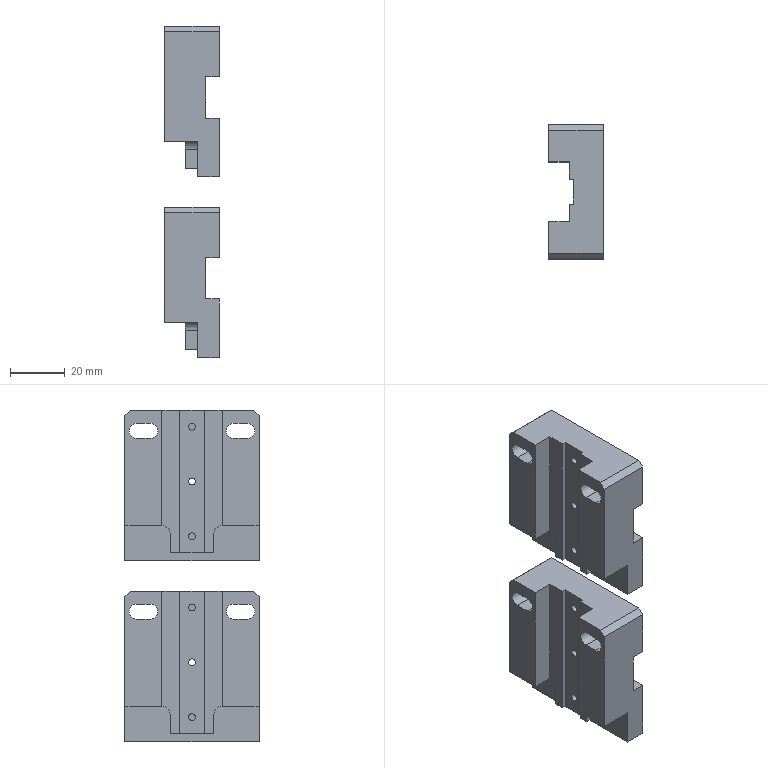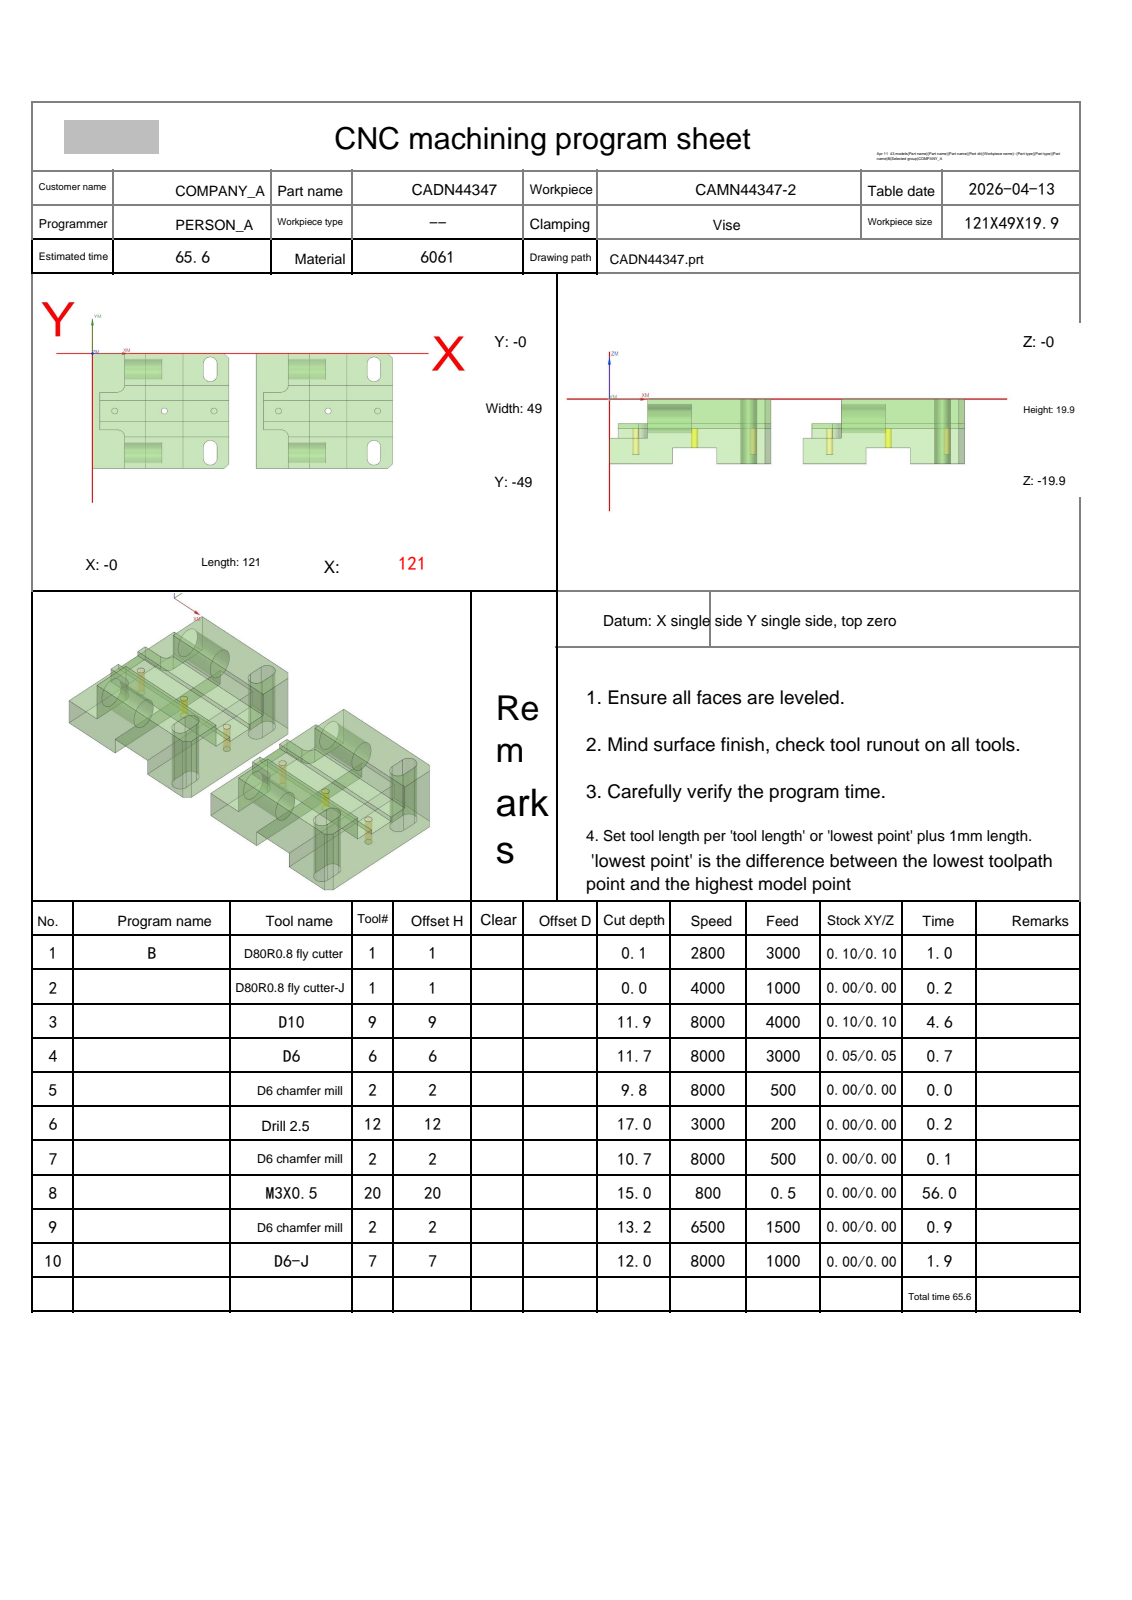NC program | NX | posted by the shop | part box 19.9 x 49 x 121 mm
Lines 3387 to 4443 of 6263:
N4 T06 M06
(D6  D=6. R=0. H=06 ce=0.10 di=0.10)
G00 G90 G54 X-3.1 Y-24.5 M03 S8000
G43 H06 Z14.902
M08
Z-6.4
G01 Z-7.9 F3000.
X.06
Y-23.05
X57.94
Y-25.95
X.06
Y-24.5
Y-24.
X-3.1
Z-6.4
G00 Y-24.5
Z-6.9
G01 Z-8.4
X.06
Y-23.05
X57.94
Y-25.95
X.06
Y-24.5
Y-24.
X-3.1
Z-6.9
G00 Y-24.5
Z-7.4
G01 Z-8.9
X.06
Y-23.05
X57.94
Y-25.95
X.06
Y-24.5
Y-24.
X-3.1
Z-7.4
G00 Z-4.4
X127.1 Y-24.5
Z-6.4
G01 Z-7.9
X123.94
Y-25.95
X66.06
Y-23.05
X123.94
Y-24.5
Y-25.
X127.1
Z-6.4
G00 Y-24.5
Z-6.9
G01 Z-8.4
X123.94
Y-25.95
X66.06
Y-23.05
X123.94
Y-24.5
Y-25.
X127.1
Z-6.9
G00 Y-24.5
Z-7.4
G01 Z-8.9
X123.94
Y-25.95
X66.06
Y-23.05
X123.94
Y-24.5
Y-25.
X127.1
Z-7.4
G00 Z14.902
G00 G90 X75.35 Y-12.85 M03 S8000
Z20.
Z-6.9
G01 X75.358 Y-12.852 Z-6.991 F2000.
X75.379 Y-12.857 Z-7.073
X75.412 Y-12.867 Z-7.147
X75.455 Y-12.88 Z-7.212
X75.506 Y-12.899 Z-7.269
X75.561 Y-12.923 Z-7.319
X75.62 Y-12.953 Z-7.361
X75.68 Y-12.989 Z-7.397
X75.739 Y-13.032 Z-7.427
X75.794 Y-13.081 Z-7.451
X75.845 Y-13.138 Z-7.47
X75.888 Y-13.204 Z-7.484
X75.921 Y-13.277 Z-7.493
X75.942 Y-13.359 Z-7.498
X75.95 Y-13.45 Z-7.5
Y-10.447
X75.934 Y-10.378 Z-7.501
X75.888 Y-10.333 Z-7.503
X75.815 Y-10.311 Z-7.506
X75.719 Y-10.31 Z-7.511
X75.603 Y-10.327 Z-7.517
X75.471 Y-10.362 Z-7.524
X75.326 Y-10.413 Z-7.531
X75.172 Y-10.477 Z-7.54
X75.011 Y-10.554 Z-7.548
X74.849 Y-10.64 Z-7.558
X74.687 Y-10.736 Z-7.568
X74.345 Y-10.969 Z-7.59
X74.026 Y-11.234 Z-7.613
X73.734 Y-11.526 Z-7.637
X73.469 Y-11.845 Z-7.66
X73.235 Y-12.187 Z-7.682
X73.14 Y-12.349 Z-7.692
X73.053 Y-12.512 Z-7.702
X72.977 Y-12.672 Z-7.71
X72.913 Y-12.826 Z-7.719
X72.862 Y-12.971 Z-7.726
X72.827 Y-13.103 Z-7.733
X72.809 Y-13.219 Z-7.739
X72.811 Y-13.315 Z-7.744
X72.833 Y-13.388 Z-7.747
X72.878 Y-13.434 Z-7.749
X72.947 Y-13.45 Z-7.75
X75.95
Y-10.447
X75.934 Y-10.378 Z-7.751
X75.888 Y-10.333 Z-7.753
X75.815 Y-10.311 Z-7.756
X75.719 Y-10.309 Z-7.761
X75.603 Y-10.327 Z-7.767
X75.471 Y-10.362 Z-7.774
X75.326 Y-10.413 Z-7.781
X75.172 Y-10.477 Z-7.79
X75.011 Y-10.553 Z-7.798
X74.849 Y-10.64 Z-7.808
X74.687 Y-10.735 Z-7.818
X74.345 Y-10.969 Z-7.84
X74.026 Y-11.234 Z-7.863
X73.734 Y-11.526 Z-7.887
X73.469 Y-11.845 Z-7.91
X73.235 Y-12.187 Z-7.932
X73.14 Y-12.349 Z-7.942
X73.053 Y-12.511 Z-7.952
X72.977 Y-12.672 Z-7.96
X72.913 Y-12.826 Z-7.969
X72.862 Y-12.971 Z-7.976
X72.827 Y-13.103 Z-7.983
X72.809 Y-13.219 Z-7.989
X72.811 Y-13.315 Z-7.994
X72.833 Y-13.388 Z-7.997
X72.878 Y-13.434 Z-7.999
X72.947 Y-13.45 Z-8.
X75.95
Y-10.447
X75.934 Y-10.378 Z-8.001
X75.888 Y-10.333 Z-8.003
X75.815 Y-10.311 Z-8.006
X75.719 Y-10.309 Z-8.011
X75.603 Y-10.327 Z-8.017
X75.471 Y-10.362 Z-8.024
X75.326 Y-10.413 Z-8.031
X75.172 Y-10.477 Z-8.04
X75.011 Y-10.553 Z-8.048
X74.849 Y-10.64 Z-8.058
X74.687 Y-10.735 Z-8.068
X74.345 Y-10.969 Z-8.09
X74.026 Y-11.234 Z-8.113
X73.734 Y-11.526 Z-8.137
X73.469 Y-11.845 Z-8.16
X73.235 Y-12.187 Z-8.182
X73.14 Y-12.349 Z-8.192
X73.053 Y-12.511 Z-8.202
X72.977 Y-12.672 Z-8.21
X72.913 Y-12.826 Z-8.219
X72.862 Y-12.971 Z-8.226
X72.827 Y-13.103 Z-8.233
X72.809 Y-13.219 Z-8.239
X72.811 Y-13.315 Z-8.244
X72.833 Y-13.388 Z-8.247
X72.878 Y-13.434 Z-8.249
X72.947 Y-13.45 Z-8.25
X75.95
Y-10.447
X75.934 Y-10.378 Z-8.251
X75.888 Y-10.333 Z-8.253
X75.815 Y-10.311 Z-8.256
X75.719 Y-10.309 Z-8.261
X75.603 Y-10.327 Z-8.267
X75.471 Y-10.362 Z-8.274
X75.326 Y-10.413 Z-8.281
X75.172 Y-10.477 Z-8.29
X75.011 Y-10.553 Z-8.298
X74.849 Y-10.64 Z-8.308
X74.687 Y-10.735 Z-8.318
X74.345 Y-10.969 Z-8.34
X74.026 Y-11.234 Z-8.363
X73.734 Y-11.526 Z-8.387
X73.469 Y-11.845 Z-8.41
X73.235 Y-12.187 Z-8.432
X73.14 Y-12.349 Z-8.442
X73.053 Y-12.511 Z-8.452
X72.977 Y-12.672 Z-8.46
X72.913 Y-12.826 Z-8.469
X72.862 Y-12.971 Z-8.476
X72.827 Y-13.103 Z-8.483
X72.809 Y-13.219 Z-8.489
X72.811 Y-13.315 Z-8.494
X72.833 Y-13.388 Z-8.497
X72.878 Y-13.434 Z-8.499
X72.947 Y-13.45 Z-8.5
X75.95
Y-10.447
X75.934 Y-10.378 Z-8.501
X75.888 Y-10.333 Z-8.503
X75.815 Y-10.311 Z-8.506
X75.719 Y-10.309 Z-8.511
X75.603 Y-10.327 Z-8.517
X75.471 Y-10.362 Z-8.524
X75.326 Y-10.413 Z-8.531
X75.172 Y-10.477 Z-8.54
X75.011 Y-10.553 Z-8.548
X74.849 Y-10.64 Z-8.558
X74.687 Y-10.735 Z-8.568
X74.345 Y-10.969 Z-8.59
X74.026 Y-11.234 Z-8.613
X73.734 Y-11.526 Z-8.637
X73.469 Y-11.845 Z-8.66
X73.235 Y-12.187 Z-8.682
X73.14 Y-12.349 Z-8.692
X73.053 Y-12.511 Z-8.702
X72.977 Y-12.672 Z-8.71
X72.913 Y-12.826 Z-8.719
X72.862 Y-12.971 Z-8.726
X72.827 Y-13.103 Z-8.733
X72.809 Y-13.219 Z-8.739
X72.811 Y-13.315 Z-8.744
X72.833 Y-13.388 Z-8.747
X72.878 Y-13.434 Z-8.749
X72.947 Y-13.45 Z-8.75
X75.95
Y-10.447
X75.934 Y-10.378 Z-8.751
X75.888 Y-10.333 Z-8.753
X75.815 Y-10.311 Z-8.756
X75.719 Y-10.309 Z-8.761
X75.603 Y-10.327 Z-8.767
X75.471 Y-10.362 Z-8.774
X75.326 Y-10.413 Z-8.781
X75.172 Y-10.477 Z-8.79
X75.011 Y-10.553 Z-8.798
X74.849 Y-10.64 Z-8.808
X74.687 Y-10.735 Z-8.818
X74.345 Y-10.969 Z-8.84
X74.026 Y-11.234 Z-8.863
X73.734 Y-11.526 Z-8.887
X73.469 Y-11.845 Z-8.91
X73.235 Y-12.187 Z-8.932
X73.14 Y-12.349 Z-8.942
X73.053 Y-12.511 Z-8.952
X72.977 Y-12.672 Z-8.96
X72.913 Y-12.826 Z-8.969
X72.862 Y-12.971 Z-8.976
X72.827 Y-13.103 Z-8.983
X72.809 Y-13.219 Z-8.989
X72.811 Y-13.315 Z-8.994
X72.833 Y-13.388 Z-8.997
X72.878 Y-13.434 Z-8.999
X72.947 Y-13.45 Z-9.
X75.95
Y-10.447
X75.934 Y-10.378 Z-9.001
X75.888 Y-10.333 Z-9.003
X75.815 Y-10.311 Z-9.006
X75.719 Y-10.309 Z-9.011
X75.603 Y-10.327 Z-9.017
X75.471 Y-10.362 Z-9.024
X75.326 Y-10.413 Z-9.031
X75.172 Y-10.477 Z-9.04
X75.011 Y-10.553 Z-9.048
X74.849 Y-10.64 Z-9.058
X74.687 Y-10.735 Z-9.068
X74.345 Y-10.969 Z-9.09
X74.026 Y-11.234 Z-9.113
X73.734 Y-11.526 Z-9.137
X73.469 Y-11.845 Z-9.16
X73.235 Y-12.187 Z-9.182
X73.14 Y-12.349 Z-9.192
X73.053 Y-12.511 Z-9.202
X72.977 Y-12.672 Z-9.21
X72.913 Y-12.826 Z-9.219
X72.862 Y-12.971 Z-9.226
X72.827 Y-13.103 Z-9.233
X72.809 Y-13.219 Z-9.239
X72.811 Y-13.315 Z-9.244
X72.833 Y-13.388 Z-9.247
X72.878 Y-13.434 Z-9.249
X72.947 Y-13.45 Z-9.25
X75.95
Y-10.447
X75.934 Y-10.378 Z-9.251
X75.888 Y-10.333 Z-9.253
X75.815 Y-10.311 Z-9.256
X75.719 Y-10.309 Z-9.261
X75.603 Y-10.327 Z-9.267
X75.471 Y-10.362 Z-9.274
X75.326 Y-10.413 Z-9.281
X75.172 Y-10.477 Z-9.29
X75.011 Y-10.553 Z-9.298
X74.849 Y-10.64 Z-9.308
X74.687 Y-10.735 Z-9.318
X74.345 Y-10.969 Z-9.34
X74.026 Y-11.234 Z-9.363
X73.734 Y-11.526 Z-9.387
X73.469 Y-11.845 Z-9.41
X73.235 Y-12.187 Z-9.432
X73.14 Y-12.349 Z-9.442
X73.053 Y-12.511 Z-9.452
X72.977 Y-12.672 Z-9.46
X72.913 Y-12.826 Z-9.469
X72.862 Y-12.971 Z-9.476
X72.827 Y-13.103 Z-9.483
X72.809 Y-13.219 Z-9.489
X72.811 Y-13.315 Z-9.494
X72.833 Y-13.388 Z-9.497
X72.878 Y-13.434 Z-9.499
X72.947 Y-13.45 Z-9.5
X75.95
Y-10.447
X75.934 Y-10.378 Z-9.501
X75.888 Y-10.333 Z-9.503
X75.815 Y-10.311 Z-9.506
X75.719 Y-10.309 Z-9.511
X75.603 Y-10.327 Z-9.517
X75.471 Y-10.362 Z-9.524
X75.326 Y-10.413 Z-9.531
X75.172 Y-10.477 Z-9.54
X75.011 Y-10.553 Z-9.548
X74.849 Y-10.64 Z-9.558
X74.687 Y-10.735 Z-9.568
X74.345 Y-10.969 Z-9.59
X74.026 Y-11.234 Z-9.613
X73.734 Y-11.526 Z-9.637
X73.469 Y-11.845 Z-9.66
X73.235 Y-12.187 Z-9.682
X73.14 Y-12.349 Z-9.692
X73.053 Y-12.511 Z-9.702
X72.977 Y-12.672 Z-9.71
X72.913 Y-12.826 Z-9.719
X72.862 Y-12.971 Z-9.726
X72.827 Y-13.103 Z-9.733
X72.809 Y-13.219 Z-9.739
X72.811 Y-13.315 Z-9.744
X72.833 Y-13.388 Z-9.747
X72.878 Y-13.434 Z-9.749
X72.947 Y-13.45 Z-9.75
X75.95
Y-10.447
X75.934 Y-10.378 Z-9.751
X75.888 Y-10.333 Z-9.753
X75.815 Y-10.311 Z-9.756
X75.719 Y-10.309 Z-9.761
X75.603 Y-10.327 Z-9.767
X75.471 Y-10.362 Z-9.774
X75.326 Y-10.413 Z-9.781
X75.172 Y-10.477 Z-9.79
X75.011 Y-10.553 Z-9.798
X74.849 Y-10.64 Z-9.808
X74.687 Y-10.735 Z-9.818
X74.345 Y-10.969 Z-9.84
X74.026 Y-11.234 Z-9.863
X73.734 Y-11.526 Z-9.887
X73.469 Y-11.845 Z-9.91
X73.235 Y-12.187 Z-9.932
X73.14 Y-12.349 Z-9.942
X73.053 Y-12.511 Z-9.952
X72.977 Y-12.672 Z-9.96
X72.913 Y-12.826 Z-9.969
X72.862 Y-12.971 Z-9.976
X72.827 Y-13.103 Z-9.983
X72.809 Y-13.219 Z-9.989
X72.811 Y-13.315 Z-9.994
X72.833 Y-13.388 Z-9.997
X72.878 Y-13.434 Z-9.999
X72.947 Y-13.45 Z-10.
X75.95
Y-10.447
X75.934 Y-10.378 Z-10.001
X75.888 Y-10.333 Z-10.003
X75.815 Y-10.311 Z-10.006
X75.719 Y-10.309 Z-10.011
X75.603 Y-10.327 Z-10.017
X75.471 Y-10.362 Z-10.024
X75.326 Y-10.413 Z-10.031
X75.172 Y-10.477 Z-10.04
X75.011 Y-10.553 Z-10.048
X74.849 Y-10.64 Z-10.058
X74.687 Y-10.735 Z-10.068
X74.345 Y-10.969 Z-10.09
X74.026 Y-11.234 Z-10.113
X73.734 Y-11.526 Z-10.137
X73.469 Y-11.845 Z-10.16
X73.235 Y-12.187 Z-10.182
X73.14 Y-12.349 Z-10.192
X73.053 Y-12.511 Z-10.202
X72.977 Y-12.672 Z-10.21
X72.913 Y-12.826 Z-10.219
X72.862 Y-12.971 Z-10.226
X72.827 Y-13.103 Z-10.233
X72.809 Y-13.219 Z-10.239
X72.811 Y-13.315 Z-10.244
X72.833 Y-13.388 Z-10.247
X72.878 Y-13.434 Z-10.249
X72.947 Y-13.45 Z-10.25
X75.95
Y-10.447
X75.934 Y-10.378 Z-10.251
X75.888 Y-10.333 Z-10.253
X75.815 Y-10.311 Z-10.256
X75.719 Y-10.309 Z-10.261
X75.603 Y-10.327 Z-10.267
X75.471 Y-10.362 Z-10.274
X75.326 Y-10.413 Z-10.281
X75.172 Y-10.477 Z-10.29
X75.011 Y-10.553 Z-10.298
X74.849 Y-10.64 Z-10.308
X74.687 Y-10.735 Z-10.318
X74.345 Y-10.969 Z-10.34
X74.026 Y-11.234 Z-10.363
X73.734 Y-11.526 Z-10.387
X73.469 Y-11.845 Z-10.41
X73.235 Y-12.187 Z-10.432
X73.14 Y-12.349 Z-10.442
X73.053 Y-12.511 Z-10.452
X72.977 Y-12.672 Z-10.46
X72.913 Y-12.826 Z-10.469
X72.862 Y-12.971 Z-10.476
X72.827 Y-13.103 Z-10.483
X72.809 Y-13.219 Z-10.489
X72.811 Y-13.315 Z-10.494
X72.833 Y-13.388 Z-10.497
X72.878 Y-13.434 Z-10.499
X72.947 Y-13.45 Z-10.5
X75.95
Y-10.447
X75.934 Y-10.378 Z-10.501
X75.888 Y-10.333 Z-10.503
X75.815 Y-10.311 Z-10.506
X75.719 Y-10.309 Z-10.511
X75.603 Y-10.327 Z-10.517
X75.471 Y-10.362 Z-10.524
X75.326 Y-10.413 Z-10.531
X75.172 Y-10.477 Z-10.54
X75.011 Y-10.553 Z-10.548
X74.849 Y-10.64 Z-10.558
X74.687 Y-10.735 Z-10.568
X74.345 Y-10.969 Z-10.59
X74.026 Y-11.234 Z-10.613
X73.734 Y-11.526 Z-10.637
X73.469 Y-11.845 Z-10.66
X73.235 Y-12.187 Z-10.682
X73.14 Y-12.349 Z-10.692
X73.053 Y-12.511 Z-10.702
X72.977 Y-12.672 Z-10.71
X72.913 Y-12.826 Z-10.719
X72.862 Y-12.971 Z-10.726
X72.827 Y-13.103 Z-10.733
X72.809 Y-13.219 Z-10.739
X72.811 Y-13.315 Z-10.744
X72.833 Y-13.388 Z-10.747
X72.878 Y-13.434 Z-10.749
X72.947 Y-13.45 Z-10.75
X75.95
Y-10.447
X75.934 Y-10.378 Z-10.751
X75.888 Y-10.333 Z-10.753
X75.815 Y-10.311 Z-10.756
X75.719 Y-10.309 Z-10.761
X75.603 Y-10.327 Z-10.767
X75.471 Y-10.362 Z-10.774
X75.326 Y-10.413 Z-10.781
X75.172 Y-10.477 Z-10.79
X75.011 Y-10.553 Z-10.798
X74.849 Y-10.64 Z-10.808
X74.687 Y-10.735 Z-10.818
X74.345 Y-10.969 Z-10.84
X74.026 Y-11.234 Z-10.863
X73.734 Y-11.526 Z-10.887
X73.469 Y-11.845 Z-10.91
X73.235 Y-12.187 Z-10.932
X73.14 Y-12.349 Z-10.942
X73.053 Y-12.511 Z-10.952
X72.977 Y-12.672 Z-10.96
X72.913 Y-12.826 Z-10.969
X72.862 Y-12.971 Z-10.976
X72.827 Y-13.103 Z-10.983
X72.809 Y-13.219 Z-10.989
X72.811 Y-13.315 Z-10.994
X72.833 Y-13.388 Z-10.997
X72.878 Y-13.434 Z-10.999
X72.947 Y-13.45 Z-11.
X75.95
Y-10.447
X75.934 Y-10.378 Z-11.001
X75.888 Y-10.333 Z-11.003
X75.815 Y-10.311 Z-11.006
X75.719 Y-10.309 Z-11.011
X75.603 Y-10.327 Z-11.017
X75.471 Y-10.362 Z-11.024
X75.326 Y-10.413 Z-11.031
X75.172 Y-10.477 Z-11.04
X75.011 Y-10.553 Z-11.048
X74.849 Y-10.64 Z-11.058
X74.687 Y-10.735 Z-11.068
X74.345 Y-10.969 Z-11.09
X74.026 Y-11.234 Z-11.113
X73.734 Y-11.526 Z-11.137
X73.469 Y-11.845 Z-11.16
X73.235 Y-12.187 Z-11.182
X73.14 Y-12.349 Z-11.192
X73.053 Y-12.511 Z-11.202
X72.977 Y-12.672 Z-11.21
X72.913 Y-12.826 Z-11.219
X72.862 Y-12.971 Z-11.226
X72.827 Y-13.103 Z-11.233
X72.809 Y-13.219 Z-11.239
X72.811 Y-13.315 Z-11.244
X72.833 Y-13.388 Z-11.247
X72.878 Y-13.434 Z-11.249
X72.947 Y-13.45 Z-11.25
X75.95
Y-10.447
X75.934 Y-10.378 Z-11.251
X75.888 Y-10.333 Z-11.253
X75.815 Y-10.311 Z-11.256
X75.719 Y-10.309 Z-11.261
X75.603 Y-10.327 Z-11.267
X75.471 Y-10.362 Z-11.274
X75.326 Y-10.413 Z-11.281
X75.172 Y-10.477 Z-11.29
X75.011 Y-10.553 Z-11.298
X74.849 Y-10.64 Z-11.308
X74.687 Y-10.735 Z-11.318
X74.345 Y-10.969 Z-11.34
X74.026 Y-11.234 Z-11.363
X73.734 Y-11.526 Z-11.387
X73.469 Y-11.845 Z-11.41
X73.235 Y-12.187 Z-11.432
X73.14 Y-12.349 Z-11.442
X73.053 Y-12.511 Z-11.452
X72.977 Y-12.672 Z-11.46
X72.913 Y-12.826 Z-11.469
X72.862 Y-12.971 Z-11.476
X72.827 Y-13.103 Z-11.483
X72.809 Y-13.219 Z-11.489
X72.811 Y-13.315 Z-11.494
X72.833 Y-13.388 Z-11.497
X72.878 Y-13.434 Z-11.499
X72.947 Y-13.45 Z-11.5
X75.95
Y-10.447
X75.934 Y-10.378 Z-11.501
X75.888 Y-10.333 Z-11.503
X75.815 Y-10.311 Z-11.506
X75.719 Y-10.309 Z-11.511
X75.603 Y-10.327 Z-11.517
X75.471 Y-10.362 Z-11.524
X75.326 Y-10.413 Z-11.531
X75.172 Y-10.477 Z-11.54
X75.011 Y-10.553 Z-11.548
X74.849 Y-10.64 Z-11.558
X74.687 Y-10.735 Z-11.568
X74.345 Y-10.969 Z-11.59
X74.026 Y-11.234 Z-11.613
X73.734 Y-11.526 Z-11.637
X73.469 Y-11.845 Z-11.66
X73.235 Y-12.187 Z-11.682
X73.14 Y-12.349 Z-11.692
X73.053 Y-12.511 Z-11.702
X72.977 Y-12.672 Z-11.71
X72.913 Y-12.826 Z-11.719
X72.862 Y-12.971 Z-11.726
X72.827 Y-13.103 Z-11.733
X72.809 Y-13.219 Z-11.739
X72.811 Y-13.315 Z-11.744
X72.833 Y-13.388 Z-11.747
X72.878 Y-13.434 Z-11.749
X72.947 Y-13.45 Z-11.75
X75.95
Y-10.447
X75.942 Y-10.356 Z-11.748
X75.921 Y-10.274 Z-11.743
X75.888 Y-10.2 Z-11.734
X75.845 Y-10.135 Z-11.72
X75.794 Y-10.078 Z-11.701
X75.739 Y-10.028 Z-11.677
X75.68 Y-9.986 Z-11.647
X75.62 Y-9.95 Z-11.611
X75.561 Y-9.92 Z-11.569
X75.506 Y-9.896 Z-11.519
X75.455 Y-9.877 Z-11.462
X75.412 Y-9.863 Z-11.397
X75.379 Y-9.854 Z-11.323
X75.358 Y-9.849 Z-11.241
X75.35 Y-9.847 Z-11.15
G00 Z3.
X75.337 Y-39.154
Z-6.9
G01 X75.345 Y-39.152 Z-6.991
X75.367 Y-39.147 Z-7.073
X75.401 Y-39.138 Z-7.147
X75.445 Y-39.124 Z-7.212
X75.496 Y-39.105 Z-7.269
X75.553 Y-39.081 Z-7.319
X75.613 Y-39.051 Z-7.361
X75.674 Y-39.015 Z-7.397
X75.734 Y-38.972 Z-7.427
X75.791 Y-38.922 Z-7.451
X75.842 Y-38.865 Z-7.47
X75.886 Y-38.8 Z-7.484
X75.92 Y-38.726 Z-7.493
X75.942 Y-38.644 Z-7.498
X75.95 Y-38.553 Z-7.5
Y-35.55
X75.937 Y-35.672 Z-7.501
X75.9 Y-35.813 Z-7.505
X75.847 Y-35.97 Z-7.512
X75.704 Y-36.327 Z-7.531
X75.56 Y-36.696 Z-7.554
X75.496 Y-36.888 Z-7.568
X75.433 Y-37.143 Z-7.586
X75.395 Y-37.393 Z-7.606
X75.381 Y-37.633 Z-7.625
X75.393 Y-37.861 Z-7.644
X75.431 Y-38.073 Z-7.664
X75.494 Y-38.265 Z-7.682
X75.543 Y-38.37 Z-7.693
X75.599 Y-38.463 Z-7.703
X75.659 Y-38.544 Z-7.713
X75.72 Y-38.61 Z-7.722
X75.779 Y-38.658 Z-7.73
X75.833 Y-38.686 Z-7.737
X75.88 Y-38.692 Z-7.742
X75.917 Y-38.673 Z-7.746
X75.941 Y-38.628 Z-7.749
X75.95 Y-38.553 Z-7.75
Y-35.55
X72.947
X72.878 Y-35.566 Z-7.751
X72.833 Y-35.612 Z-7.753
X72.811 Y-35.685 Z-7.756
X72.809 Y-35.781 Z-7.761
X72.826 Y-35.897 Z-7.767
X72.861 Y-36.029 Z-7.774
X72.911 Y-36.174 Z-7.781
X72.975 Y-36.328 Z-7.79
X73.051 Y-36.489 Z-7.798
X73.137 Y-36.652 Z-7.808
X73.232 Y-36.814 Z-7.818
X73.465 Y-37.156 Z-7.84
X73.728 Y-37.474 Z-7.863
X74.02 Y-37.767 Z-7.887
X74.338 Y-38.031 Z-7.91
X74.68 Y-38.265 Z-7.932
X74.843 Y-38.361 Z-7.942
X75.006 Y-38.447 Z-7.952
X75.167 Y-38.524 Z-7.96
X75.322 Y-38.588 Z-7.969
X75.468 Y-38.638 Z-7.976
X75.601 Y-38.673 Z-7.983
X75.717 Y-38.691 Z-7.989
X75.814 Y-38.689 Z-7.994
X75.887 Y-38.667 Z-7.997
X75.934 Y-38.622 Z-7.999
X75.95 Y-38.553 Z-8.
Y-35.55
X72.947
X72.878 Y-35.566 Z-8.001
X72.833 Y-35.612 Z-8.003
X72.811 Y-35.685 Z-8.006
X72.809 Y-35.781 Z-8.011
X72.826 Y-35.897 Z-8.017
X72.861 Y-36.029 Z-8.024
X72.911 Y-36.174 Z-8.031
X72.975 Y-36.328 Z-8.04
X73.051 Y-36.489 Z-8.048
X73.137 Y-36.652 Z-8.058
X73.232 Y-36.814 Z-8.068
X73.465 Y-37.156 Z-8.09
X73.728 Y-37.474 Z-8.113
X74.02 Y-37.767 Z-8.137
X74.338 Y-38.031 Z-8.16
X74.68 Y-38.265 Z-8.182
X74.843 Y-38.361 Z-8.192
X75.006 Y-38.447 Z-8.202
X75.167 Y-38.524 Z-8.21
X75.322 Y-38.588 Z-8.219
X75.468 Y-38.638 Z-8.226
X75.601 Y-38.673 Z-8.233
X75.717 Y-38.691 Z-8.239
X75.814 Y-38.689 Z-8.244
X75.887 Y-38.667 Z-8.247
X75.934 Y-38.622 Z-8.249
X75.95 Y-38.553 Z-8.25
Y-35.55
X72.947
X72.878 Y-35.566 Z-8.251
X72.833 Y-35.612 Z-8.253
X72.811 Y-35.685 Z-8.256
X72.809 Y-35.781 Z-8.261
X72.826 Y-35.897 Z-8.267
X72.861 Y-36.029 Z-8.274
X72.911 Y-36.174 Z-8.281
X72.975 Y-36.328 Z-8.29
X73.051 Y-36.489 Z-8.298
X73.137 Y-36.652 Z-8.308
X73.232 Y-36.814 Z-8.318
X73.465 Y-37.156 Z-8.34
X73.728 Y-37.474 Z-8.363
X74.02 Y-37.767 Z-8.387
X74.338 Y-38.031 Z-8.41
X74.68 Y-38.265 Z-8.432
X74.843 Y-38.361 Z-8.442
X75.006 Y-38.447 Z-8.452
X75.167 Y-38.524 Z-8.46
X75.322 Y-38.588 Z-8.469
X75.468 Y-38.638 Z-8.476
X75.601 Y-38.673 Z-8.483
X75.717 Y-38.691 Z-8.489
X75.814 Y-38.689 Z-8.494
X75.887 Y-38.667 Z-8.497
X75.934 Y-38.622 Z-8.499
X75.95 Y-38.553 Z-8.5
Y-35.55
X72.947
X72.878 Y-35.566 Z-8.501
X72.833 Y-35.612 Z-8.503
X72.811 Y-35.685 Z-8.506
X72.809 Y-35.781 Z-8.511
X72.826 Y-35.897 Z-8.517
X72.861 Y-36.029 Z-8.524
X72.911 Y-36.174 Z-8.531
X72.975 Y-36.328 Z-8.54
X73.051 Y-36.489 Z-8.548
X73.137 Y-36.652 Z-8.558
X73.232 Y-36.814 Z-8.568
X73.465 Y-37.156 Z-8.59
X73.728 Y-37.474 Z-8.613
X74.02 Y-37.767 Z-8.637
X74.338 Y-38.031 Z-8.66
X74.68 Y-38.265 Z-8.682
X74.843 Y-38.361 Z-8.692
X75.006 Y-38.447 Z-8.702
X75.167 Y-38.524 Z-8.71
X75.322 Y-38.588 Z-8.719
X75.468 Y-38.638 Z-8.726
X75.601 Y-38.673 Z-8.733
X75.717 Y-38.691 Z-8.739
X75.814 Y-38.689 Z-8.744
X75.887 Y-38.667 Z-8.747
X75.934 Y-38.622 Z-8.749
X75.95 Y-38.553 Z-8.75
Y-35.55
X72.947
X72.878 Y-35.566 Z-8.751
X72.833 Y-35.612 Z-8.753
X72.811 Y-35.685 Z-8.756
X72.809 Y-35.781 Z-8.761
X72.826 Y-35.897 Z-8.767
X72.861 Y-36.029 Z-8.774
X72.911 Y-36.174 Z-8.781
X72.975 Y-36.328 Z-8.79
X73.051 Y-36.489 Z-8.798
X73.137 Y-36.652 Z-8.808
X73.232 Y-36.814 Z-8.818
X73.465 Y-37.156 Z-8.84
X73.728 Y-37.474 Z-8.863
X74.02 Y-37.767 Z-8.887
X74.338 Y-38.031 Z-8.91
X74.68 Y-38.265 Z-8.932
X74.843 Y-38.361 Z-8.942
X75.006 Y-38.447 Z-8.952
X75.167 Y-38.524 Z-8.96
X75.322 Y-38.588 Z-8.969
X75.468 Y-38.638 Z-8.976
X75.601 Y-38.673 Z-8.983
X75.717 Y-38.691 Z-8.989
X75.814 Y-38.689 Z-8.994
X75.887 Y-38.667 Z-8.997
X75.934 Y-38.622 Z-8.999
X75.95 Y-38.553 Z-9.
Y-35.55
X72.947
X72.878 Y-35.566 Z-9.001
X72.833 Y-35.612 Z-9.003
X72.811 Y-35.685 Z-9.006
X72.809 Y-35.781 Z-9.011
X72.826 Y-35.897 Z-9.017
X72.861 Y-36.029 Z-9.024
X72.911 Y-36.174 Z-9.031
X72.975 Y-36.328 Z-9.04
X73.051 Y-36.489 Z-9.048
X73.137 Y-36.652 Z-9.058
X73.232 Y-36.814 Z-9.068
X73.465 Y-37.156 Z-9.09
X73.728 Y-37.474 Z-9.113
X74.02 Y-37.767 Z-9.137
X74.338 Y-38.031 Z-9.16
X74.68 Y-38.265 Z-9.182
X74.843 Y-38.361 Z-9.192
X75.006 Y-38.447 Z-9.202
X75.167 Y-38.524 Z-9.21
X75.322 Y-38.588 Z-9.219
X75.468 Y-38.638 Z-9.226
X75.601 Y-38.673 Z-9.233
X75.717 Y-38.691 Z-9.239
X75.814 Y-38.689 Z-9.244
X75.887 Y-38.667 Z-9.247
X75.934 Y-38.622 Z-9.249
X75.95 Y-38.553 Z-9.25
Y-35.55
X72.947
X72.878 Y-35.566 Z-9.251
X72.833 Y-35.612 Z-9.253
X72.811 Y-35.685 Z-9.256
X72.809 Y-35.781 Z-9.261
X72.826 Y-35.897 Z-9.267
X72.861 Y-36.029 Z-9.274
X72.911 Y-36.174 Z-9.281
X72.975 Y-36.328 Z-9.29
X73.051 Y-36.489 Z-9.298
X73.137 Y-36.652 Z-9.308
X73.232 Y-36.814 Z-9.318
X73.465 Y-37.156 Z-9.34
X73.728 Y-37.474 Z-9.363
X74.02 Y-37.767 Z-9.387
X74.338 Y-38.031 Z-9.41
X74.68 Y-38.265 Z-9.432
X74.843 Y-38.361 Z-9.442
X75.006 Y-38.447 Z-9.452
X75.167 Y-38.524 Z-9.46
X75.322 Y-38.588 Z-9.469
X75.468 Y-38.638 Z-9.476
X75.601 Y-38.673 Z-9.483
X75.717 Y-38.691 Z-9.489
X75.814 Y-38.689 Z-9.494
X75.887 Y-38.667 Z-9.497
X75.934 Y-38.622 Z-9.499
X75.95 Y-38.553 Z-9.5
Y-35.55
X72.947
X72.878 Y-35.566 Z-9.501
X72.833 Y-35.612 Z-9.503
X72.811 Y-35.685 Z-9.506
X72.809 Y-35.781 Z-9.511
X72.826 Y-35.897 Z-9.517
X72.861 Y-36.029 Z-9.524
X72.911 Y-36.174 Z-9.531
X72.975 Y-36.328 Z-9.54
X73.051 Y-36.489 Z-9.548
X73.137 Y-36.652 Z-9.558
X73.232 Y-36.814 Z-9.568
X73.465 Y-37.156 Z-9.59
X73.728 Y-37.474 Z-9.613
X74.02 Y-37.767 Z-9.637
X74.338 Y-38.031 Z-9.66
X74.68 Y-38.265 Z-9.682
X74.843 Y-38.361 Z-9.692
X75.006 Y-38.447 Z-9.702
X75.167 Y-38.524 Z-9.71
X75.322 Y-38.588 Z-9.719
X75.468 Y-38.638 Z-9.726
X75.601 Y-38.673 Z-9.733
X75.717 Y-38.691 Z-9.739
X75.814 Y-38.689 Z-9.744
X75.887 Y-38.667 Z-9.747
X75.934 Y-38.622 Z-9.749
X75.95 Y-38.553 Z-9.75
Y-35.55
X72.947
X72.878 Y-35.566 Z-9.751
X72.833 Y-35.612 Z-9.753
X72.811 Y-35.685 Z-9.756
X72.809 Y-35.781 Z-9.761
X72.826 Y-35.897 Z-9.767
X72.861 Y-36.029 Z-9.774
X72.911 Y-36.174 Z-9.781
X72.975 Y-36.328 Z-9.79
X73.051 Y-36.489 Z-9.798
X73.137 Y-36.652 Z-9.808
X73.232 Y-36.814 Z-9.818
X73.465 Y-37.156 Z-9.84
X73.728 Y-37.474 Z-9.863
X74.02 Y-37.767 Z-9.887
X74.338 Y-38.031 Z-9.91
X74.68 Y-38.265 Z-9.932
X74.843 Y-38.361 Z-9.942
X75.006 Y-38.447 Z-9.952
X75.167 Y-38.524 Z-9.96
X75.322 Y-38.588 Z-9.969
X75.468 Y-38.638 Z-9.976
X75.601 Y-38.673 Z-9.983
X75.717 Y-38.691 Z-9.989
X75.814 Y-38.689 Z-9.994
X75.887 Y-38.667 Z-9.997
X75.934 Y-38.622 Z-9.999
X75.95 Y-38.553 Z-10.
Y-35.55
X72.947
X72.878 Y-35.566 Z-10.001
X72.833 Y-35.612 Z-10.003
X72.811 Y-35.685 Z-10.006
X72.809 Y-35.781 Z-10.011
X72.826 Y-35.897 Z-10.017
X72.861 Y-36.029 Z-10.024
X72.911 Y-36.174 Z-10.031
X72.975 Y-36.328 Z-10.04
X73.051 Y-36.489 Z-10.048
X73.137 Y-36.652 Z-10.058
X73.232 Y-36.814 Z-10.068
X73.465 Y-37.156 Z-10.09
X73.728 Y-37.474 Z-10.113
X74.02 Y-37.767 Z-10.137
X74.338 Y-38.031 Z-10.16
X74.68 Y-38.265 Z-10.182
X74.843 Y-38.361 Z-10.192
X75.006 Y-38.447 Z-10.202
X75.167 Y-38.524 Z-10.21
X75.322 Y-38.588 Z-10.219
X75.468 Y-38.638 Z-10.226
X75.601 Y-38.673 Z-10.233
X75.717 Y-38.691 Z-10.239
X75.814 Y-38.689 Z-10.244
X75.887 Y-38.667 Z-10.247
X75.934 Y-38.622 Z-10.249
X75.95 Y-38.553 Z-10.25
Y-35.55
X72.947
X72.878 Y-35.566 Z-10.251
X72.833 Y-35.612 Z-10.253
X72.811 Y-35.685 Z-10.256
X72.809 Y-35.781 Z-10.261
X72.826 Y-35.897 Z-10.267
X72.861 Y-36.029 Z-10.274
X72.911 Y-36.174 Z-10.281
X72.975 Y-36.328 Z-10.29
X73.051 Y-36.489 Z-10.298
X73.137 Y-36.652 Z-10.308
X73.232 Y-36.814 Z-10.318
X73.465 Y-37.156 Z-10.34
X73.728 Y-37.474 Z-10.363
X74.02 Y-37.767 Z-10.387
X74.338 Y-38.031 Z-10.41
X74.68 Y-38.265 Z-10.432
X74.843 Y-38.361 Z-10.442
X75.006 Y-38.447 Z-10.452
X75.167 Y-38.524 Z-10.46
X75.322 Y-38.588 Z-10.469
X75.468 Y-38.638 Z-10.476
X75.601 Y-38.673 Z-10.483
X75.717 Y-38.691 Z-10.489
X75.814 Y-38.689 Z-10.494
X75.887 Y-38.667 Z-10.497
X75.934 Y-38.622 Z-10.499
X75.95 Y-38.553 Z-10.5
Y-35.55
X72.947
X72.878 Y-35.566 Z-10.501
X72.833 Y-35.612 Z-10.503
X72.811 Y-35.685 Z-10.506
X72.809 Y-35.781 Z-10.511
X72.826 Y-35.897 Z-10.517
X72.861 Y-36.029 Z-10.524
X72.911 Y-36.174 Z-10.531
X72.975 Y-36.328 Z-10.54
X73.051 Y-36.489 Z-10.548
X73.137 Y-36.652 Z-10.558
X73.232 Y-36.814 Z-10.568
X73.465 Y-37.156 Z-10.59
X73.728 Y-37.474 Z-10.613
X74.02 Y-37.767 Z-10.637
X74.338 Y-38.031 Z-10.66
X74.68 Y-38.265 Z-10.682
X74.843 Y-38.361 Z-10.692
X75.006 Y-38.447 Z-10.702
X75.167 Y-38.524 Z-10.71
X75.322 Y-38.588 Z-10.719
X75.468 Y-38.638 Z-10.726
X75.601 Y-38.673 Z-10.733
X75.717 Y-38.691 Z-10.739
X75.814 Y-38.689 Z-10.744
X75.887 Y-38.667 Z-10.747
X75.934 Y-38.622 Z-10.749
X75.95 Y-38.553 Z-10.75
Y-35.55
X72.947
X72.878 Y-35.566 Z-10.751
X72.833 Y-35.612 Z-10.753
X72.811 Y-35.685 Z-10.756
X72.809 Y-35.781 Z-10.761
X72.826 Y-35.897 Z-10.767
X72.861 Y-36.029 Z-10.774
X72.911 Y-36.174 Z-10.781
X72.975 Y-36.328 Z-10.79
X73.051 Y-36.489 Z-10.798
X73.137 Y-36.652 Z-10.808
X73.232 Y-36.814 Z-10.818
X73.465 Y-37.156 Z-10.84
X73.728 Y-37.474 Z-10.863
X74.02 Y-37.767 Z-10.887
X74.338 Y-38.031 Z-10.91
X74.68 Y-38.265 Z-10.932
X74.843 Y-38.361 Z-10.942
X75.006 Y-38.447 Z-10.952
X75.167 Y-38.524 Z-10.96
X75.322 Y-38.588 Z-10.969
X75.468 Y-38.638 Z-10.976
X75.601 Y-38.673 Z-10.983
X75.717 Y-38.691 Z-10.989
X75.814 Y-38.689 Z-10.994
X75.887 Y-38.667 Z-10.997
X75.934 Y-38.622 Z-10.999
X75.95 Y-38.553 Z-11.
Y-35.55
X72.947
X72.878 Y-35.566 Z-11.001
X72.833 Y-35.612 Z-11.003
X72.811 Y-35.685 Z-11.006
X72.809 Y-35.781 Z-11.011
X72.826 Y-35.897 Z-11.017
X72.861 Y-36.029 Z-11.024
X72.911 Y-36.174 Z-11.031
X72.975 Y-36.328 Z-11.04
X73.051 Y-36.489 Z-11.048
X73.137 Y-36.652 Z-11.058
X73.232 Y-36.814 Z-11.068
X73.465 Y-37.156 Z-11.09
X73.728 Y-37.474 Z-11.113
X74.02 Y-37.767 Z-11.137
X74.338 Y-38.031 Z-11.16
X74.68 Y-38.265 Z-11.182
X74.843 Y-38.361 Z-11.192
X75.006 Y-38.447 Z-11.202
X75.167 Y-38.524 Z-11.21
X75.322 Y-38.588 Z-11.219
X75.468 Y-38.638 Z-11.226
X75.601 Y-38.673 Z-11.233
X75.717 Y-38.691 Z-11.239
X75.814 Y-38.689 Z-11.244
X75.887 Y-38.667 Z-11.247
X75.934 Y-38.622 Z-11.249
X75.95 Y-38.553 Z-11.25
Y-35.55
X72.947
X72.878 Y-35.566 Z-11.251
X72.833 Y-35.612 Z-11.253
X72.811 Y-35.685 Z-11.256